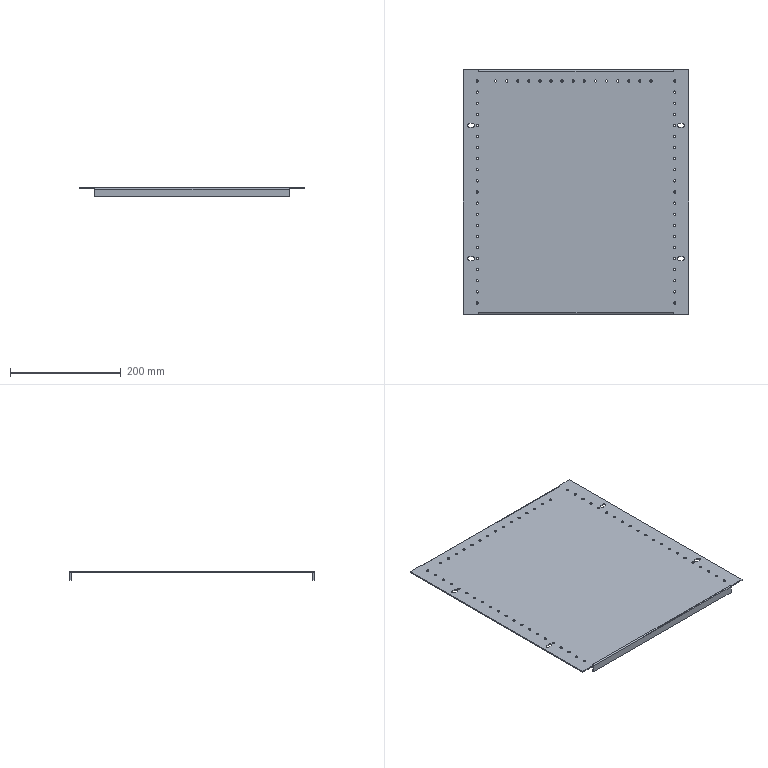Part | SolidWorks | features ICE 5, MoveFace 4, BaseBody 1 | 1 solid | 164 faces | box 406 x 440 x 15 mm | volume 372648 mm3 | cylinder 130 | plane 34 | commonest cylinder face diameters 4.2 x116 7 x12 0.2 x2